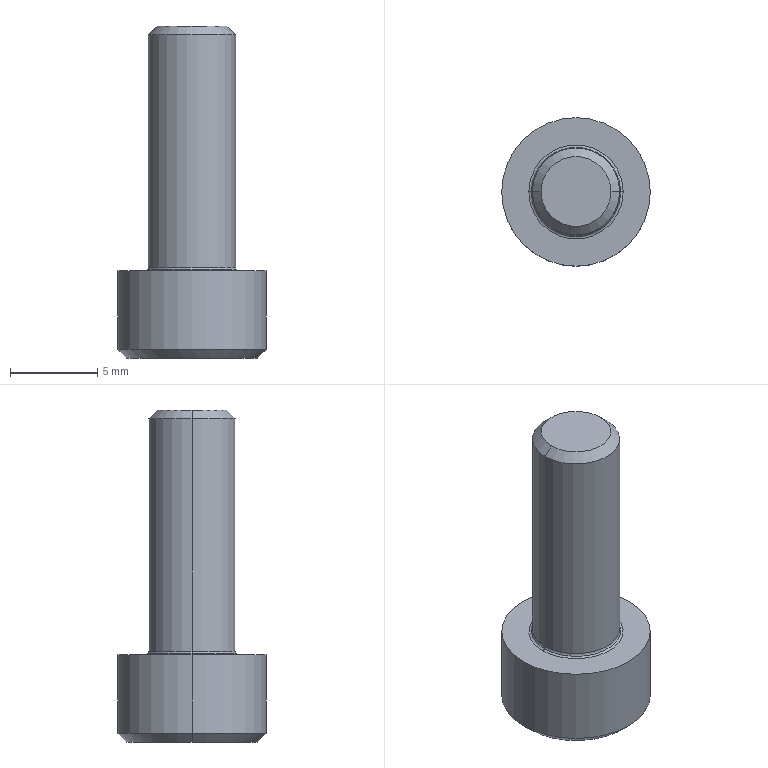Part | Creo | 1 solid | 23 faces | box 8.5 x 8.5 x 19 mm | volume 511.829 mm3 | plane 9 | cone 6 | cylinder 4 | torus 4 | commonest cylinder face diameters 5 x2 8.5 x2
STEP:
#1=CARTESIAN_POINT('',(307.691,256.,-7.5));
#2=VERTEX_POINT('',#1);
#3=CARTESIAN_POINT('',(308.845,258.,-7.5));
#4=VERTEX_POINT('',#3);
#5=CARTESIAN_POINT('',(307.691,256.,-7.5));
#6=CARTESIAN_POINT('',(307.744,256.093,-7.469));
#7=CARTESIAN_POINT('',(307.852,256.28,-7.413));
#8=CARTESIAN_POINT('',(308.018,256.567,-7.352));
#9=CARTESIAN_POINT('',(308.185,256.856,-7.32));
#10=CARTESIAN_POINT('',(308.352,257.146,-7.32));
#11=CARTESIAN_POINT('',(308.519,257.435,-7.352));
#12=CARTESIAN_POINT('',(308.684,257.721,-7.413));
#13=CARTESIAN_POINT('',(308.792,257.907,-7.469));
#14=CARTESIAN_POINT('',(308.845,258.,-7.5));
#15=B_SPLINE_CURVE_WITH_KNOTS('',3,(#5,#6,#7,#8,#9,#10,#11,#12,#13,#14),.UNSPECIFIED.,.F.,.F.,(4,1,1,1,1,1,1,4),(0.,0.1429,0.2857,0.4286,0.5714,0.7143,0.8571,1.),.UNSPECIFIED.);
#16=EDGE_CURVE('',#2,#4,#15,.T.);
#17=ORIENTED_EDGE('',*,*,#16,.F.);
#18=CARTESIAN_POINT('',(310.,256.,-6.167));
#19=VERTEX_POINT('',#18);
#20=CARTESIAN_POINT('',(310.,256.,-6.167));
#21=DIRECTION('',(-0.866,0.,-0.5));
#22=VECTOR('',#21,2.667);
#23=LINE('',#20,#22);
#24=EDGE_CURVE('',#19,#2,#23,.T.);
#25=ORIENTED_EDGE('',*,*,#24,.F.);
#26=CARTESIAN_POINT('',(312.309,256.,-7.5));
#27=VERTEX_POINT('',#26);
#28=CARTESIAN_POINT('',(310.,256.,-6.167));
#29=DIRECTION('',(0.866,0.,-0.5));
#30=VECTOR('',#29,2.667);
#31=LINE('',#28,#30);
#32=EDGE_CURVE('',#19,#27,#31,.T.);
#33=ORIENTED_EDGE('',*,*,#32,.T.);
#34=CARTESIAN_POINT('',(311.155,258.,-7.5));
#35=VERTEX_POINT('',#34);
#36=CARTESIAN_POINT('',(311.155,258.,-7.5));
#37=CARTESIAN_POINT('',(311.208,257.907,-7.469));
#38=CARTESIAN_POINT('',(311.317,257.72,-7.413));
#39=CARTESIAN_POINT('',(311.482,257.433,-7.352));
#40=CARTESIAN_POINT('',(311.649,257.144,-7.32));
#41=CARTESIAN_POINT('',(311.816,256.854,-7.32));
#42=CARTESIAN_POINT('',(311.983,256.565,-7.352));
#43=CARTESIAN_POINT('',(312.148,256.279,-7.413));
#44=CARTESIAN_POINT('',(312.256,256.093,-7.469));
#45=CARTESIAN_POINT('',(312.309,256.,-7.5));
#46=B_SPLINE_CURVE_WITH_KNOTS('',3,(#36,#37,#38,#39,#40,#41,#42,#43,#44,#45),.UNSPECIFIED.,.F.,.F.,(4,1,1,1,1,1,1,4),(0.,0.1429,0.2857,0.4286,0.5714,0.7143,0.8571,1.),.UNSPECIFIED.);
#47=EDGE_CURVE('',#35,#27,#46,.T.);
#48=ORIENTED_EDGE('',*,*,#47,.F.);
#49=CARTESIAN_POINT('',(308.845,258.,-7.5));
#50=CARTESIAN_POINT('',(308.908,258.,-7.482));
#51=CARTESIAN_POINT('',(309.03,258.,-7.449));
#52=CARTESIAN_POINT('',(309.207,258.,-7.408));
#53=CARTESIAN_POINT('',(309.381,258.,-7.374));
#54=CARTESIAN_POINT('',(309.555,258.,-7.348));
#55=CARTESIAN_POINT('',(309.732,258.,-7.33));
#56=CARTESIAN_POINT('',(309.91,258.,-7.321));
#57=CARTESIAN_POINT('',(310.09,258.,-7.321));
#58=CARTESIAN_POINT('',(310.268,258.,-7.33));
#59=CARTESIAN_POINT('',(310.445,258.,-7.348));
#60=CARTESIAN_POINT('',(310.619,258.,-7.374));
#61=CARTESIAN_POINT('',(310.793,258.,-7.408));
#62=CARTESIAN_POINT('',(310.97,258.,-7.449));
#63=CARTESIAN_POINT('',(311.092,258.,-7.482));
#64=CARTESIAN_POINT('',(311.155,258.,-7.5));
#65=B_SPLINE_CURVE_WITH_KNOTS('',3,(#49,#50,#51,#52,#53,#54,#55,#56,#57,#58,#59,#60,#61,#62,#63,#64),.UNSPECIFIED.,.F.,.F.,(4,1,1,1,1,1,1,1,1,1,1,1,1,4),(0.,0.07692,0.1538,0.2308,0.3077,0.3846,0.4615,0.5385,0.6154,0.6923,0.7692,0.8462,0.9231,1.),.UNSPECIFIED.);
#66=EDGE_CURVE('',#4,#35,#65,.T.);
#67=ORIENTED_EDGE('',*,*,#66,.F.);
#68=EDGE_LOOP('',(#17,#25,#33,#48,#67));
#69=FACE_OUTER_BOUND('',#68,.F.);
#70=CARTESIAN_POINT('',(310.,256.,-6.847));
#71=DIRECTION('',(0.,0.,-1.));
#72=DIRECTION('',(-1.,0.,0.));
#73=AXIS2_PLACEMENT_3D('',#70,#71,#72);
#74=CONICAL_SURFACE('',#73,1.178,60.);
#75=ADVANCED_FACE('',(#69),#74,.F.);
#76=CARTESIAN_POINT('',(308.845,258.,-10.));
#77=VERTEX_POINT('',#76);
#78=CARTESIAN_POINT('',(307.691,256.,-10.));
#79=VERTEX_POINT('',#78);
#80=CARTESIAN_POINT('',(308.845,258.,-10.));
#81=DIRECTION('',(-0.5,-0.866,0.));
#82=VECTOR('',#81,2.309);
#83=LINE('',#80,#82);
#84=EDGE_CURVE('',#77,#79,#83,.T.);
#85=ORIENTED_EDGE('',*,*,#84,.T.);
#86=CARTESIAN_POINT('',(307.691,256.,-10.));
#87=DIRECTION('',(0.,0.,1.));
#88=VECTOR('',#87,2.5);
#89=LINE('',#86,#88);
#90=EDGE_CURVE('',#79,#2,#89,.T.);
#91=ORIENTED_EDGE('',*,*,#90,.T.);
#92=ORIENTED_EDGE('',*,*,#16,.T.);
#93=CARTESIAN_POINT('',(308.845,258.,-10.));
#94=DIRECTION('',(0.,0.,1.));
#95=VECTOR('',#94,2.5);
#96=LINE('',#93,#95);
#97=EDGE_CURVE('',#77,#4,#96,.T.);
#98=ORIENTED_EDGE('',*,*,#97,.F.);
#99=EDGE_LOOP('',(#85,#91,#92,#98));
#100=FACE_OUTER_BOUND('',#99,.F.);
#101=CARTESIAN_POINT('',(308.845,258.,-7.5));
#102=DIRECTION('',(0.866,-0.5,0.));
#103=DIRECTION('',(-0.5,-0.866,0.));
#104=AXIS2_PLACEMENT_3D('',#101,#102,#103);
#105=PLANE('',#104);
#106=ADVANCED_FACE('',(#100),#105,.T.);
#107=CARTESIAN_POINT('',(306.25,256.,-10.));
#108=VERTEX_POINT('',#107);
#109=CARTESIAN_POINT('',(313.75,256.,-10.));
#110=VERTEX_POINT('',#109);
#111=CARTESIAN_POINT('',(310.,256.,-10.));
#112=DIRECTION('',(0.,0.,-1.));
#113=DIRECTION('',(-1.,0.,0.));
#114=AXIS2_PLACEMENT_3D('',#111,#112,#113);
#115=CIRCLE('',#114,3.75);
#116=EDGE_CURVE('',#108,#110,#115,.T.);
#117=ORIENTED_EDGE('',*,*,#116,.F.);
#118=CARTESIAN_POINT('',(310.,256.,-10.));
#119=DIRECTION('',(0.,0.,-1.));
#120=DIRECTION('',(1.,0.,0.));
#121=AXIS2_PLACEMENT_3D('',#118,#119,#120);
#122=CIRCLE('',#121,3.75);
#123=EDGE_CURVE('',#110,#108,#122,.T.);
#124=ORIENTED_EDGE('',*,*,#123,.F.);
#125=EDGE_LOOP('',(#117,#124));
#126=FACE_OUTER_BOUND('',#125,.F.);
#127=CARTESIAN_POINT('',(308.845,254.,-10.));
#128=VERTEX_POINT('',#127);
#129=CARTESIAN_POINT('',(307.691,256.,-10.));
#130=DIRECTION('',(0.5,-0.866,0.));
#131=VECTOR('',#130,2.309);
#132=LINE('',#129,#131);
#133=EDGE_CURVE('',#79,#128,#132,.T.);
#134=ORIENTED_EDGE('',*,*,#133,.F.);
#135=ORIENTED_EDGE('',*,*,#84,.F.);
#136=CARTESIAN_POINT('',(311.155,258.,-10.));
#137=VERTEX_POINT('',#136);
#138=CARTESIAN_POINT('',(308.845,258.,-10.));
#139=DIRECTION('',(1.,0.,0.));
#140=VECTOR('',#139,2.309);
#141=LINE('',#138,#140);
#142=EDGE_CURVE('',#77,#137,#141,.T.);
#143=ORIENTED_EDGE('',*,*,#142,.T.);
#144=CARTESIAN_POINT('',(312.309,256.,-10.));
#145=VERTEX_POINT('',#144);
#146=CARTESIAN_POINT('',(312.309,256.,-10.));
#147=DIRECTION('',(-0.5,0.866,0.));
#148=VECTOR('',#147,2.309);
#149=LINE('',#146,#148);
#150=EDGE_CURVE('',#145,#137,#149,.T.);
#151=ORIENTED_EDGE('',*,*,#150,.F.);
#152=CARTESIAN_POINT('',(311.155,254.,-10.));
#153=VERTEX_POINT('',#152);
#154=CARTESIAN_POINT('',(311.155,254.,-10.));
#155=DIRECTION('',(0.5,0.866,0.));
#156=VECTOR('',#155,2.309);
#157=LINE('',#154,#156);
#158=EDGE_CURVE('',#153,#145,#157,.T.);
#159=ORIENTED_EDGE('',*,*,#158,.F.);
#160=CARTESIAN_POINT('',(311.155,254.,-10.));
#161=DIRECTION('',(-1.,0.,0.));
#162=VECTOR('',#161,2.309);
#163=LINE('',#160,#162);
#164=EDGE_CURVE('',#153,#128,#163,.T.);
#165=ORIENTED_EDGE('',*,*,#164,.T.);
#166=EDGE_LOOP('',(#134,#135,#143,#151,#159,#165));
#167=FACE_BOUND('',#166,.F.);
#168=CARTESIAN_POINT('',(310.,256.,-10.));
#169=DIRECTION('',(0.,0.,-1.));
#170=DIRECTION('',(-1.,0.,0.));
#171=AXIS2_PLACEMENT_3D('',#168,#169,#170);
#172=PLANE('',#171);
#173=ADVANCED_FACE('',(#126,#167),#172,.T.);
#174=CARTESIAN_POINT('',(305.75,256.,-9.5));
#175=VERTEX_POINT('',#174);
#176=CARTESIAN_POINT('',(314.25,256.,-9.5));
#177=VERTEX_POINT('',#176);
#178=CARTESIAN_POINT('',(310.,256.,-9.5));
#179=DIRECTION('',(0.,0.,-1.));
#180=DIRECTION('',(-1.,0.,0.));
#181=AXIS2_PLACEMENT_3D('',#178,#179,#180);
#182=CIRCLE('',#181,4.25);
#183=EDGE_CURVE('',#175,#177,#182,.T.);
#184=ORIENTED_EDGE('',*,*,#183,.F.);
#185=CARTESIAN_POINT('',(306.25,256.,-10.));
#186=DIRECTION('',(-0.7071,0.,0.7071));
#187=VECTOR('',#186,0.7071);
#188=LINE('',#185,#187);
#189=EDGE_CURVE('',#108,#175,#188,.T.);
#190=ORIENTED_EDGE('',*,*,#189,.F.);
#191=ORIENTED_EDGE('',*,*,#116,.T.);
#192=CARTESIAN_POINT('',(313.75,256.,-10.));
#193=DIRECTION('',(0.7071,0.,0.7071));
#194=VECTOR('',#193,0.7071);
#195=LINE('',#192,#194);
#196=EDGE_CURVE('',#110,#177,#195,.T.);
#197=ORIENTED_EDGE('',*,*,#196,.T.);
#198=EDGE_LOOP('',(#184,#190,#191,#197));
#199=FACE_OUTER_BOUND('',#198,.F.);
#200=CARTESIAN_POINT('',(310.,256.,-9.75));
#201=DIRECTION('',(0.,0.,1.));
#202=DIRECTION('',(1.,0.,0.));
#203=AXIS2_PLACEMENT_3D('',#200,#201,#202);
#204=CONICAL_SURFACE('',#203,4.,45.);
#205=ADVANCED_FACE('',(#199),#204,.T.);
#206=ORIENTED_EDGE('',*,*,#183,.T.);
#207=CARTESIAN_POINT('',(314.25,256.,-5.));
#208=VERTEX_POINT('',#207);
#209=CARTESIAN_POINT('',(314.25,256.,-5.));
#210=DIRECTION('',(0.,0.,-1.));
#211=VECTOR('',#210,4.5);
#212=LINE('',#209,#211);
#213=EDGE_CURVE('',#208,#177,#212,.T.);
#214=ORIENTED_EDGE('',*,*,#213,.F.);
#215=CARTESIAN_POINT('',(305.75,256.,-5.));
#216=VERTEX_POINT('',#215);
#217=CARTESIAN_POINT('',(310.,256.,-5.));
#218=DIRECTION('',(0.,0.,1.));
#219=DIRECTION('',(1.,0.,0.));
#220=AXIS2_PLACEMENT_3D('',#217,#218,#219);
#221=CIRCLE('',#220,4.25);
#222=EDGE_CURVE('',#208,#216,#221,.T.);
#223=ORIENTED_EDGE('',*,*,#222,.T.);
#224=CARTESIAN_POINT('',(305.75,256.,-5.));
#225=DIRECTION('',(0.,0.,-1.));
#226=VECTOR('',#225,4.5);
#227=LINE('',#224,#226);
#228=EDGE_CURVE('',#216,#175,#227,.T.);
#229=ORIENTED_EDGE('',*,*,#228,.T.);
#230=EDGE_LOOP('',(#206,#214,#223,#229));
#231=FACE_OUTER_BOUND('',#230,.F.);
#232=CARTESIAN_POINT('',(310.,256.,-5.));
#233=DIRECTION('',(0.,0.,-1.));
#234=DIRECTION('',(-1.,0.,0.));
#235=AXIS2_PLACEMENT_3D('',#232,#233,#234);
#236=CYLINDRICAL_SURFACE('',#235,4.25);
#237=ADVANCED_FACE('',(#231),#236,.T.);
#238=CARTESIAN_POINT('',(310.,256.,-9.5));
#239=DIRECTION('',(0.,0.,-1.));
#240=DIRECTION('',(1.,0.,0.));
#241=AXIS2_PLACEMENT_3D('',#238,#239,#240);
#242=CIRCLE('',#241,4.25);
#243=EDGE_CURVE('',#177,#175,#242,.T.);
#244=ORIENTED_EDGE('',*,*,#243,.T.);
#245=ORIENTED_EDGE('',*,*,#228,.F.);
#246=CARTESIAN_POINT('',(310.,256.,-5.));
#247=DIRECTION('',(0.,0.,1.));
#248=DIRECTION('',(-1.,0.,0.));
#249=AXIS2_PLACEMENT_3D('',#246,#247,#248);
#250=CIRCLE('',#249,4.25);
#251=EDGE_CURVE('',#216,#208,#250,.T.);
#252=ORIENTED_EDGE('',*,*,#251,.T.);
#253=ORIENTED_EDGE('',*,*,#213,.T.);
#254=EDGE_LOOP('',(#244,#245,#252,#253));
#255=FACE_OUTER_BOUND('',#254,.F.);
#256=CARTESIAN_POINT('',(310.,256.,-5.));
#257=DIRECTION('',(0.,0.,-1.));
#258=DIRECTION('',(-1.,0.,0.));
#259=AXIS2_PLACEMENT_3D('',#256,#257,#258);
#260=CYLINDRICAL_SURFACE('',#259,4.25);
#261=ADVANCED_FACE('',(#255),#260,.T.);
#262=ORIENTED_EDGE('',*,*,#243,.F.);
#263=ORIENTED_EDGE('',*,*,#196,.F.);
#264=ORIENTED_EDGE('',*,*,#123,.T.);
#265=ORIENTED_EDGE('',*,*,#189,.T.);
#266=EDGE_LOOP('',(#262,#263,#264,#265));
#267=FACE_OUTER_BOUND('',#266,.F.);
#268=CARTESIAN_POINT('',(310.,256.,-9.75));
#269=DIRECTION('',(0.,0.,1.));
#270=DIRECTION('',(1.,0.,0.));
#271=AXIS2_PLACEMENT_3D('',#268,#269,#270);
#272=CONICAL_SURFACE('',#271,4.,45.);
#273=ADVANCED_FACE('',(#267),#272,.T.);
#274=ORIENTED_EDGE('',*,*,#251,.F.);
#275=ORIENTED_EDGE('',*,*,#222,.F.);
#276=EDGE_LOOP('',(#274,#275));
#277=FACE_OUTER_BOUND('',#276,.F.);
#278=CARTESIAN_POINT('',(307.3,256.,-5.));
#279=VERTEX_POINT('',#278);
#280=CARTESIAN_POINT('',(312.7,256.,-5.));
#281=VERTEX_POINT('',#280);
#282=CARTESIAN_POINT('',(310.,256.,-5.));
#283=DIRECTION('',(0.,0.,-1.));
#284=DIRECTION('',(-1.,0.,0.));
#285=AXIS2_PLACEMENT_3D('',#282,#283,#284);
#286=CIRCLE('',#285,2.7);
#287=EDGE_CURVE('',#279,#281,#286,.T.);
#288=ORIENTED_EDGE('',*,*,#287,.F.);
#289=CARTESIAN_POINT('',(310.,256.,-5.));
#290=DIRECTION('',(0.,0.,-1.));
#291=DIRECTION('',(1.,0.,0.));
#292=AXIS2_PLACEMENT_3D('',#289,#290,#291);
#293=CIRCLE('',#292,2.7);
#294=EDGE_CURVE('',#281,#279,#293,.T.);
#295=ORIENTED_EDGE('',*,*,#294,.F.);
#296=EDGE_LOOP('',(#288,#295));
#297=FACE_BOUND('',#296,.F.);
#298=CARTESIAN_POINT('',(310.,256.,-5.));
#299=DIRECTION('',(0.,0.,-1.));
#300=DIRECTION('',(-1.,0.,0.));
#301=AXIS2_PLACEMENT_3D('',#298,#299,#300);
#302=PLANE('',#301);
#303=ADVANCED_FACE('',(#277,#297),#302,.F.);
#304=ORIENTED_EDGE('',*,*,#287,.T.);
#305=CARTESIAN_POINT('',(312.559,256.,-4.941));
#306=VERTEX_POINT('',#305);
#307=CARTESIAN_POINT('',(312.7,256.,-4.8));
#308=DIRECTION('',(0.,1.,0.));
#309=DIRECTION('',(0.,0.,-1.));
#310=AXIS2_PLACEMENT_3D('',#307,#308,#309);
#311=CIRCLE('',#310,0.2);
#312=EDGE_CURVE('',#281,#306,#311,.T.);
#313=ORIENTED_EDGE('',*,*,#312,.T.);
#314=CARTESIAN_POINT('',(307.441,256.,-4.941));
#315=VERTEX_POINT('',#314);
#316=CARTESIAN_POINT('',(310.,256.,-4.941));
#317=DIRECTION('',(0.,0.,-1.));
#318=DIRECTION('',(-1.,0.,0.));
#319=AXIS2_PLACEMENT_3D('',#316,#317,#318);
#320=CIRCLE('',#319,2.559);
#321=EDGE_CURVE('',#315,#306,#320,.T.);
#322=ORIENTED_EDGE('',*,*,#321,.F.);
#323=CARTESIAN_POINT('',(307.3,256.,-4.8));
#324=DIRECTION('',(0.,-1.,0.));
#325=DIRECTION('',(0.,0.,-1.));
#326=AXIS2_PLACEMENT_3D('',#323,#324,#325);
#327=CIRCLE('',#326,0.2);
#328=EDGE_CURVE('',#279,#315,#327,.T.);
#329=ORIENTED_EDGE('',*,*,#328,.F.);
#330=EDGE_LOOP('',(#304,#313,#322,#329));
#331=FACE_OUTER_BOUND('',#330,.F.);
#332=CARTESIAN_POINT('',(310.,256.,-4.8));
#333=DIRECTION('',(0.,0.,-1.));
#334=DIRECTION('',(-1.,0.,0.));
#335=AXIS2_PLACEMENT_3D('',#332,#333,#334);
#336=TOROIDAL_SURFACE('',#335,2.7,0.2);
#337=ADVANCED_FACE('',(#331),#336,.F.);
#338=ORIENTED_EDGE('',*,*,#294,.T.);
#339=ORIENTED_EDGE('',*,*,#328,.T.);
#340=CARTESIAN_POINT('',(310.,256.,-4.941));
#341=DIRECTION('',(0.,0.,-1.));
#342=DIRECTION('',(1.,0.,0.));
#343=AXIS2_PLACEMENT_3D('',#340,#341,#342);
#344=CIRCLE('',#343,2.559);
#345=EDGE_CURVE('',#306,#315,#344,.T.);
#346=ORIENTED_EDGE('',*,*,#345,.F.);
#347=ORIENTED_EDGE('',*,*,#312,.F.);
#348=EDGE_LOOP('',(#338,#339,#346,#347));
#349=FACE_OUTER_BOUND('',#348,.F.);
#350=CARTESIAN_POINT('',(310.,256.,-4.8));
#351=DIRECTION('',(0.,0.,-1.));
#352=DIRECTION('',(-1.,0.,0.));
#353=AXIS2_PLACEMENT_3D('',#350,#351,#352);
#354=TOROIDAL_SURFACE('',#353,2.7,0.2);
#355=ADVANCED_FACE('',(#349),#354,.F.);
#356=CARTESIAN_POINT('',(312.5,256.,-4.8));
#357=VERTEX_POINT('',#356);
#358=CARTESIAN_POINT('',(307.5,256.,-4.8));
#359=VERTEX_POINT('',#358);
#360=CARTESIAN_POINT('',(310.,256.,-4.8));
#361=DIRECTION('',(0.,0.,-1.));
#362=DIRECTION('',(1.,0.,0.));
#363=AXIS2_PLACEMENT_3D('',#360,#361,#362);
#364=CIRCLE('',#363,2.5);
#365=EDGE_CURVE('',#357,#359,#364,.T.);
#366=ORIENTED_EDGE('',*,*,#365,.F.);
#367=CARTESIAN_POINT('',(312.7,256.,-4.8));
#368=DIRECTION('',(0.,1.,0.));
#369=DIRECTION('',(-0.7071,0.,-0.7071));
#370=AXIS2_PLACEMENT_3D('',#367,#368,#369);
#371=CIRCLE('',#370,0.2);
#372=EDGE_CURVE('',#306,#357,#371,.T.);
#373=ORIENTED_EDGE('',*,*,#372,.F.);
#374=ORIENTED_EDGE('',*,*,#345,.T.);
#375=CARTESIAN_POINT('',(307.3,256.,-4.8));
#376=DIRECTION('',(0.,-1.,0.));
#377=DIRECTION('',(0.7071,0.,-0.7071));
#378=AXIS2_PLACEMENT_3D('',#375,#376,#377);
#379=CIRCLE('',#378,0.2);
#380=EDGE_CURVE('',#315,#359,#379,.T.);
#381=ORIENTED_EDGE('',*,*,#380,.T.);
#382=EDGE_LOOP('',(#366,#373,#374,#381));
#383=FACE_OUTER_BOUND('',#382,.F.);
#384=CARTESIAN_POINT('',(310.,256.,-4.8));
#385=DIRECTION('',(0.,0.,-1.));
#386=DIRECTION('',(-1.,0.,0.));
#387=AXIS2_PLACEMENT_3D('',#384,#385,#386);
#388=TOROIDAL_SURFACE('',#387,2.7,0.2);
#389=ADVANCED_FACE('',(#383),#388,.F.);
#390=CARTESIAN_POINT('',(307.5,256.,8.5));
#391=VERTEX_POINT('',#390);
#392=CARTESIAN_POINT('',(312.5,256.,8.5));
#393=VERTEX_POINT('',#392);
#394=CARTESIAN_POINT('',(310.,256.,8.5));
#395=DIRECTION('',(0.,0.,1.));
#396=DIRECTION('',(-1.,0.,0.));
#397=AXIS2_PLACEMENT_3D('',#394,#395,#396);
#398=CIRCLE('',#397,2.5);
#399=EDGE_CURVE('',#391,#393,#398,.T.);
#400=ORIENTED_EDGE('',*,*,#399,.T.);
#401=CARTESIAN_POINT('',(312.5,256.,8.5));
#402=DIRECTION('',(0.,0.,-1.));
#403=VECTOR('',#402,13.3);
#404=LINE('',#401,#403);
#405=EDGE_CURVE('',#393,#357,#404,.T.);
#406=ORIENTED_EDGE('',*,*,#405,.T.);
#407=ORIENTED_EDGE('',*,*,#365,.T.);
#408=CARTESIAN_POINT('',(307.5,256.,8.5));
#409=DIRECTION('',(0.,0.,-1.));
#410=VECTOR('',#409,13.3);
#411=LINE('',#408,#410);
#412=EDGE_CURVE('',#391,#359,#411,.T.);
#413=ORIENTED_EDGE('',*,*,#412,.F.);
#414=EDGE_LOOP('',(#400,#406,#407,#413));
#415=FACE_OUTER_BOUND('',#414,.F.);
#416=CARTESIAN_POINT('',(310.,256.,9.));
#417=DIRECTION('',(0.,0.,-1.));
#418=DIRECTION('',(-1.,0.,0.));
#419=AXIS2_PLACEMENT_3D('',#416,#417,#418);
#420=CYLINDRICAL_SURFACE('',#419,2.5);
#421=ADVANCED_FACE('',(#415),#420,.T.);
#422=CARTESIAN_POINT('',(308.,256.,9.));
#423=VERTEX_POINT('',#422);
#424=CARTESIAN_POINT('',(312.,256.,9.));
#425=VERTEX_POINT('',#424);
#426=CARTESIAN_POINT('',(310.,256.,9.));
#427=DIRECTION('',(0.,0.,1.));
#428=DIRECTION('',(-1.,0.,0.));
#429=AXIS2_PLACEMENT_3D('',#426,#427,#428);
#430=CIRCLE('',#429,2.);
#431=EDGE_CURVE('',#423,#425,#430,.T.);
#432=ORIENTED_EDGE('',*,*,#431,.T.);
#433=CARTESIAN_POINT('',(312.,256.,9.));
#434=DIRECTION('',(0.7071,0.,-0.7071));
#435=VECTOR('',#434,0.7071);
#436=LINE('',#433,#435);
#437=EDGE_CURVE('',#425,#393,#436,.T.);
#438=ORIENTED_EDGE('',*,*,#437,.T.);
#439=ORIENTED_EDGE('',*,*,#399,.F.);
#440=CARTESIAN_POINT('',(308.,256.,9.));
#441=DIRECTION('',(-0.7071,0.,-0.7071));
#442=VECTOR('',#441,0.7071);
#443=LINE('',#440,#442);
#444=EDGE_CURVE('',#423,#391,#443,.T.);
#445=ORIENTED_EDGE('',*,*,#444,.F.);
#446=EDGE_LOOP('',(#432,#438,#439,#445));
#447=FACE_OUTER_BOUND('',#446,.F.);
#448=CARTESIAN_POINT('',(310.,256.,8.75));
#449=DIRECTION('',(0.,0.,-1.));
#450=DIRECTION('',(-1.,0.,0.));
#451=AXIS2_PLACEMENT_3D('',#448,#449,#450);
#452=CONICAL_SURFACE('',#451,2.25,45.);
#453=ADVANCED_FACE('',(#447),#452,.T.);
#454=ORIENTED_EDGE('',*,*,#431,.F.);
#455=CARTESIAN_POINT('',(310.,256.,9.));
#456=DIRECTION('',(0.,0.,1.));
#457=DIRECTION('',(1.,0.,0.));
#458=AXIS2_PLACEMENT_3D('',#455,#456,#457);
#459=CIRCLE('',#458,2.);
#460=EDGE_CURVE('',#425,#423,#459,.T.);
#461=ORIENTED_EDGE('',*,*,#460,.F.);
#462=EDGE_LOOP('',(#454,#461));
#463=FACE_OUTER_BOUND('',#462,.F.);
#464=CARTESIAN_POINT('',(310.,256.,9.));
#465=DIRECTION('',(0.,0.,-1.));
#466=DIRECTION('',(-1.,0.,0.));
#467=AXIS2_PLACEMENT_3D('',#464,#465,#466);
#468=PLANE('',#467);
#469=ADVANCED_FACE('',(#463),#468,.F.);
#470=ORIENTED_EDGE('',*,*,#460,.T.);
#471=ORIENTED_EDGE('',*,*,#444,.T.);
#472=CARTESIAN_POINT('',(310.,256.,8.5));
#473=DIRECTION('',(0.,0.,1.));
#474=DIRECTION('',(1.,0.,0.));
#475=AXIS2_PLACEMENT_3D('',#472,#473,#474);
#476=CIRCLE('',#475,2.5);
#477=EDGE_CURVE('',#393,#391,#476,.T.);
#478=ORIENTED_EDGE('',*,*,#477,.F.);
#479=ORIENTED_EDGE('',*,*,#437,.F.);
#480=EDGE_LOOP('',(#470,#471,#478,#479));
#481=FACE_OUTER_BOUND('',#480,.F.);
#482=CARTESIAN_POINT('',(310.,256.,8.75));
#483=DIRECTION('',(0.,0.,-1.));
#484=DIRECTION('',(-1.,0.,0.));
#485=AXIS2_PLACEMENT_3D('',#482,#483,#484);
#486=CONICAL_SURFACE('',#485,2.25,45.);
#487=ADVANCED_FACE('',(#481),#486,.T.);
#488=ORIENTED_EDGE('',*,*,#477,.T.);
#489=ORIENTED_EDGE('',*,*,#412,.T.);
#490=CARTESIAN_POINT('',(310.,256.,-4.8));
#491=DIRECTION('',(0.,0.,-1.));
#492=DIRECTION('',(-1.,0.,0.));
#493=AXIS2_PLACEMENT_3D('',#490,#491,#492);
#494=CIRCLE('',#493,2.5);
#495=EDGE_CURVE('',#359,#357,#494,.T.);
#496=ORIENTED_EDGE('',*,*,#495,.T.);
#497=ORIENTED_EDGE('',*,*,#405,.F.);
#498=EDGE_LOOP('',(#488,#489,#496,#497));
#499=FACE_OUTER_BOUND('',#498,.F.);
#500=CARTESIAN_POINT('',(310.,256.,9.));
#501=DIRECTION('',(0.,0.,-1.));
#502=DIRECTION('',(-1.,0.,0.));
#503=AXIS2_PLACEMENT_3D('',#500,#501,#502);
#504=CYLINDRICAL_SURFACE('',#503,2.5);
#505=ADVANCED_FACE('',(#499),#504,.T.);
#506=ORIENTED_EDGE('',*,*,#495,.F.);
#507=ORIENTED_EDGE('',*,*,#380,.F.);
#508=ORIENTED_EDGE('',*,*,#321,.T.);
#509=ORIENTED_EDGE('',*,*,#372,.T.);
#510=EDGE_LOOP('',(#506,#507,#508,#509));
#511=FACE_OUTER_BOUND('',#510,.F.);
#512=CARTESIAN_POINT('',(310.,256.,-4.8));
#513=DIRECTION('',(0.,0.,-1.));
#514=DIRECTION('',(-1.,0.,0.));
#515=AXIS2_PLACEMENT_3D('',#512,#513,#514);
#516=TOROIDAL_SURFACE('',#515,2.7,0.2);
#517=ADVANCED_FACE('',(#511),#516,.F.);
#518=ORIENTED_EDGE('',*,*,#133,.T.);
#519=CARTESIAN_POINT('',(308.845,254.,-7.5));
#520=VERTEX_POINT('',#519);
#521=CARTESIAN_POINT('',(308.845,254.,-10.));
#522=DIRECTION('',(0.,0.,1.));
#523=VECTOR('',#522,2.5);
#524=LINE('',#521,#523);
#525=EDGE_CURVE('',#128,#520,#524,.T.);
#526=ORIENTED_EDGE('',*,*,#525,.T.);
#527=CARTESIAN_POINT('',(308.845,254.,-7.5));
#528=CARTESIAN_POINT('',(308.792,254.093,-7.469));
#529=CARTESIAN_POINT('',(308.683,254.28,-7.413));
#530=CARTESIAN_POINT('',(308.518,254.567,-7.352));
#531=CARTESIAN_POINT('',(308.351,254.856,-7.32));
#532=CARTESIAN_POINT('',(308.184,255.146,-7.32));
#533=CARTESIAN_POINT('',(308.017,255.435,-7.352));
#534=CARTESIAN_POINT('',(307.852,255.721,-7.413));
#535=CARTESIAN_POINT('',(307.744,255.907,-7.469));
#536=CARTESIAN_POINT('',(307.691,256.,-7.5));
#537=B_SPLINE_CURVE_WITH_KNOTS('',3,(#527,#528,#529,#530,#531,#532,#533,#534,#535,#536),.UNSPECIFIED.,.F.,.F.,(4,1,1,1,1,1,1,4),(0.,0.1429,0.2857,0.4286,0.5714,0.7143,0.8571,1.),.UNSPECIFIED.);
#538=EDGE_CURVE('',#520,#2,#537,.T.);
#539=ORIENTED_EDGE('',*,*,#538,.T.);
#540=ORIENTED_EDGE('',*,*,#90,.F.);
#541=EDGE_LOOP('',(#518,#526,#539,#540));
#542=FACE_OUTER_BOUND('',#541,.F.);
#543=CARTESIAN_POINT('',(307.691,256.,-7.5));
#544=DIRECTION('',(0.866,0.5,0.));
#545=DIRECTION('',(0.5,-0.866,0.));
#546=AXIS2_PLACEMENT_3D('',#543,#544,#545);
#547=PLANE('',#546);
#548=ADVANCED_FACE('',(#542),#547,.T.);
#549=ORIENTED_EDGE('',*,*,#164,.F.);
#550=CARTESIAN_POINT('',(311.155,254.,-7.5));
#551=VERTEX_POINT('',#550);
#552=CARTESIAN_POINT('',(311.155,254.,-10.));
#553=DIRECTION('',(0.,0.,1.));
#554=VECTOR('',#553,2.5);
#555=LINE('',#552,#554);
#556=EDGE_CURVE('',#153,#551,#555,.T.);
#557=ORIENTED_EDGE('',*,*,#556,.T.);
#558=CARTESIAN_POINT('',(311.155,254.,-7.5));
#559=CARTESIAN_POINT('',(311.092,254.,-7.482));
#560=CARTESIAN_POINT('',(310.97,254.,-7.449));
#561=CARTESIAN_POINT('',(310.793,254.,-7.408));
#562=CARTESIAN_POINT('',(310.619,254.,-7.374));
#563=CARTESIAN_POINT('',(310.445,254.,-7.348));
#564=CARTESIAN_POINT('',(310.268,254.,-7.33));
#565=CARTESIAN_POINT('',(310.09,254.,-7.321));
#566=CARTESIAN_POINT('',(309.91,254.,-7.321));
#567=CARTESIAN_POINT('',(309.732,254.,-7.33));
#568=CARTESIAN_POINT('',(309.555,254.,-7.348));
#569=CARTESIAN_POINT('',(309.381,254.,-7.374));
#570=CARTESIAN_POINT('',(309.207,254.,-7.408));
#571=CARTESIAN_POINT('',(309.03,254.,-7.449));
#572=CARTESIAN_POINT('',(308.908,254.,-7.482));
#573=CARTESIAN_POINT('',(308.845,254.,-7.5));
#574=B_SPLINE_CURVE_WITH_KNOTS('',3,(#558,#559,#560,#561,#562,#563,#564,#565,#566,#567,#568,#569,#570,#571,#572,#573),.UNSPECIFIED.,.F.,.F.,(4,1,1,1,1,1,1,1,1,1,1,1,1,4),(0.,0.07692,0.1538,0.2308,0.3077,0.3846,0.4615,0.5385,0.6154,0.6923,0.7692,0.8462,0.9231,1.),.UNSPECIFIED.);
#575=EDGE_CURVE('',#551,#520,#574,.T.);
#576=ORIENTED_EDGE('',*,*,#575,.T.);
#577=ORIENTED_EDGE('',*,*,#525,.F.);
#578=EDGE_LOOP('',(#549,#557,#576,#577));
#579=FACE_OUTER_BOUND('',#578,.F.);
#580=CARTESIAN_POINT('',(308.845,254.,-7.5));
#581=DIRECTION('',(0.,1.,0.));
#582=DIRECTION('',(0.,0.,-1.));
#583=AXIS2_PLACEMENT_3D('',#580,#581,#582);
#584=PLANE('',#583);
#585=ADVANCED_FACE('',(#579),#584,.T.);
#586=ORIENTED_EDGE('',*,*,#158,.T.);
#587=CARTESIAN_POINT('',(312.309,256.,-10.));
#588=DIRECTION('',(0.,0.,1.));
#589=VECTOR('',#588,2.5);
#590=LINE('',#587,#589);
#591=EDGE_CURVE('',#145,#27,#590,.T.);
#592=ORIENTED_EDGE('',*,*,#591,.T.);
#593=CARTESIAN_POINT('',(312.309,256.,-7.5));
#594=CARTESIAN_POINT('',(312.256,255.907,-7.469));
#595=CARTESIAN_POINT('',(312.148,255.721,-7.413));
#596=CARTESIAN_POINT('',(311.983,255.435,-7.352));
#597=CARTESIAN_POINT('',(311.816,255.146,-7.32));
#598=CARTESIAN_POINT('',(311.649,254.856,-7.32));
#599=CARTESIAN_POINT('',(311.482,254.567,-7.352));
#600=CARTESIAN_POINT('',(311.317,254.28,-7.413));
#601=CARTESIAN_POINT('',(311.208,254.093,-7.469));
#602=CARTESIAN_POINT('',(311.155,254.,-7.5));
#603=B_SPLINE_CURVE_WITH_KNOTS('',3,(#593,#594,#595,#596,#597,#598,#599,#600,#601,#602),.UNSPECIFIED.,.F.,.F.,(4,1,1,1,1,1,1,4),(0.,0.1429,0.2857,0.4286,0.5714,0.7143,0.8571,1.),.UNSPECIFIED.);
#604=EDGE_CURVE('',#27,#551,#603,.T.);
#605=ORIENTED_EDGE('',*,*,#604,.T.);
#606=ORIENTED_EDGE('',*,*,#556,.F.);
#607=EDGE_LOOP('',(#586,#592,#605,#606));
#608=FACE_OUTER_BOUND('',#607,.F.);
#609=CARTESIAN_POINT('',(311.155,254.,-7.5));
#610=DIRECTION('',(-0.866,0.5,0.));
#611=DIRECTION('',(0.5,0.866,0.));
#612=AXIS2_PLACEMENT_3D('',#609,#610,#611);
#613=PLANE('',#612);
#614=ADVANCED_FACE('',(#608),#613,.T.);
#615=ORIENTED_EDGE('',*,*,#150,.T.);
#616=CARTESIAN_POINT('',(311.155,258.,-10.));
#617=DIRECTION('',(0.,0.,1.));
#618=VECTOR('',#617,2.5);
#619=LINE('',#616,#618);
#620=EDGE_CURVE('',#137,#35,#619,.T.);
#621=ORIENTED_EDGE('',*,*,#620,.T.);
#622=ORIENTED_EDGE('',*,*,#47,.T.);
#623=ORIENTED_EDGE('',*,*,#591,.F.);
#624=EDGE_LOOP('',(#615,#621,#622,#623));
#625=FACE_OUTER_BOUND('',#624,.F.);
#626=CARTESIAN_POINT('',(312.309,256.,-7.5));
#627=DIRECTION('',(-0.866,-0.5,0.));
#628=DIRECTION('',(-0.5,0.866,0.));
#629=AXIS2_PLACEMENT_3D('',#626,#627,#628);
#630=PLANE('',#629);
#631=ADVANCED_FACE('',(#625),#630,.T.);
#632=ORIENTED_EDGE('',*,*,#142,.F.);
#633=ORIENTED_EDGE('',*,*,#97,.T.);
#634=ORIENTED_EDGE('',*,*,#66,.T.);
#635=ORIENTED_EDGE('',*,*,#620,.F.);
#636=EDGE_LOOP('',(#632,#633,#634,#635));
#637=FACE_OUTER_BOUND('',#636,.F.);
#638=CARTESIAN_POINT('',(311.155,258.,-7.5));
#639=DIRECTION('',(0.,-1.,0.));
#640=DIRECTION('',(0.,0.,1.));
#641=AXIS2_PLACEMENT_3D('',#638,#639,#640);
#642=PLANE('',#641);
#643=ADVANCED_FACE('',(#637),#642,.T.);
#644=ORIENTED_EDGE('',*,*,#604,.F.);
#645=ORIENTED_EDGE('',*,*,#32,.F.);
#646=ORIENTED_EDGE('',*,*,#24,.T.);
#647=ORIENTED_EDGE('',*,*,#538,.F.);
#648=ORIENTED_EDGE('',*,*,#575,.F.);
#649=EDGE_LOOP('',(#644,#645,#646,#647,#648));
#650=FACE_OUTER_BOUND('',#649,.F.);
#651=CARTESIAN_POINT('',(310.,256.,-6.847));
#652=DIRECTION('',(0.,0.,-1.));
#653=DIRECTION('',(-1.,0.,0.));
#654=AXIS2_PLACEMENT_3D('',#651,#652,#653);
#655=CONICAL_SURFACE('',#654,1.178,60.);
#656=ADVANCED_FACE('',(#650),#655,.F.);
#657=CLOSED_SHELL('',(#75,#106,#173,#205,#237,#261,#273,#303,#337,#355,#389,#421,#453,#469,#487,#505,#517,#548,#585,#614,#631,#643,#656));
#658=MANIFOLD_SOLID_BREP('',#657);
#659=(LENGTH_UNIT()NAMED_UNIT(*)SI_UNIT(.MILLI.,.METRE.));
#660=UNCERTAINTY_MEASURE_WITH_UNIT(LENGTH_MEASURE(0.002248),#659,'','');
#661=(NAMED_UNIT(*)PLANE_ANGLE_UNIT()SI_UNIT($,.RADIAN.));
#662=PLANE_ANGLE_MEASURE_WITH_UNIT(PLANE_ANGLE_MEASURE(0.01745),#661);
#663=(CONVERSION_BASED_UNIT('DEGREE',#662)NAMED_UNIT(*)PLANE_ANGLE_UNIT());
#664=(NAMED_UNIT(*)SI_UNIT($,.STERADIAN.)SOLID_ANGLE_UNIT());
#665=(GEOMETRIC_REPRESENTATION_CONTEXT(3)GLOBAL_UNCERTAINTY_ASSIGNED_CONTEXT((#660))GLOBAL_UNIT_ASSIGNED_CONTEXT((#659,#663,#664))REPRESENTATION_CONTEXT('',''));
#666=ADVANCED_BREP_SHAPE_REPRESENTATION('',(#658),#665);